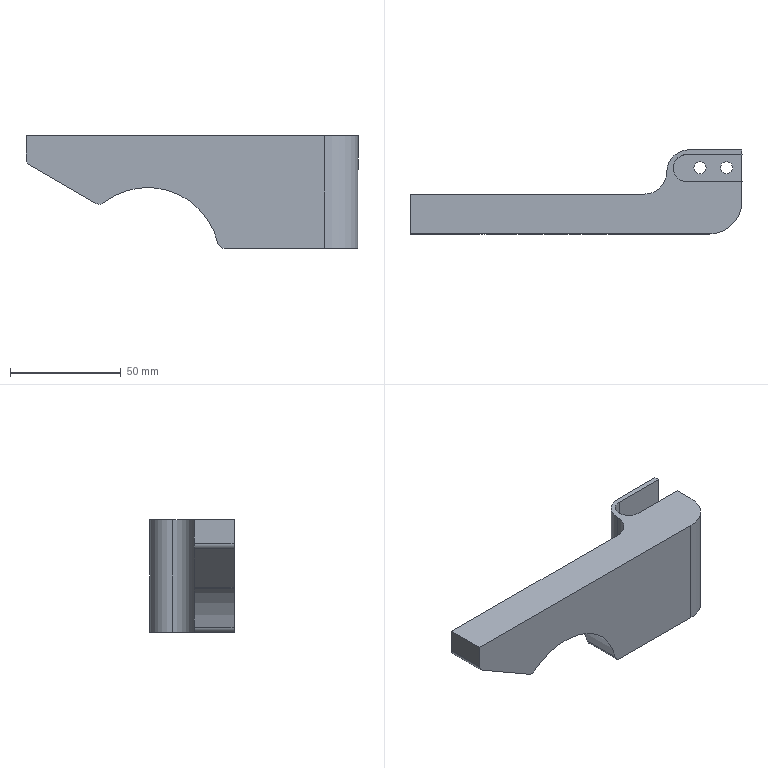CAM job | NX | 3-axis milling, drilling | part box 150 x 38 x 51 mm | stock box 160 x 48 x 52 mm
Tools:
number,name,description,diameter,corner_radius,flute_length,length,flutes
1,D63,Milling Tool-5 Parameters,63.0,0.0,50.0,75.0,2
12,D12C,Milling Tool-5 Parameters,12.0,0.0,50.0,75.0,2
8,R4,Milling Tool-5 Parameters,8.0,4.0,50.0,75.0,2
7,D6A45,Milling Tool-5 Parameters,6.0,0.0,50.0,75.0,2
15,5.5ZT,Drilling Tool,5.5,0.0,35.0,50.0,2
6,D6,Milling Tool-5 Parameters,6.0,0.0,50.0,75.0,2
11,D12JING,Milling Tool-5 Parameters,12.0,0.0,50.0,75.0,2
Operations:
program,operation,operation_type,tool,method,geometry_group,spindle_rpm,surface_speed,feed_per_tooth,feed_cut,feed_plunge,cut_length_mm,path_length_mm,cut_time_min,machine_time_min
1,FLOOR_WALL,VolumeBased25DMillingOperation,D63,METHOD,A,6500.0,1286.0,0.1154,1500.0,100.0,480.797,534.797,0.3205,0.3259
1,DRILLING,Operation,D6A45,METHOD,A,5000.0,94.0,0.025,250.0,0.0,8.0,91.369,0.032,0.0403
1,DRILLING_COPY,Operation,5.5ZT,METHOD,A,2000.0,34.0,0.05,200.0,0.0,89.305,253.979,0.4465,0.463
1,ADAPTIVE_MILLING,CavityMilling,D12C,METHOD,A,9500.0,358.0,0.1579,3000.0,1000.0,5698.893,5804.893,1.902,1.912
1,ADAPTIVE_MILLING_COPY,CavityMilling,D12C,METHOD,A,9500.0,358.0,0.1579,3000.0,1000.0,5696.238,5852.238,1.901,1.916
1,CAVITY_MILL,CavityMilling,D12C,METHOD,A,9500.0,358.0,0.1316,2500.0,1000.0,10840.921,11390.241,4.866,4.921
1,ZLEVEL_PROFILE_COPY_COPY_COPY_1_COPY_COPY_COPY,ZLevelMilling,D12JING,METHOD,A,9500.0,358.0,0.0632,1200.0,1000.0,1630.857,1796.09,1.362,1.378
1,HOLE_MILLING,CylinderMilling,D6,METHOD,A,9500.0,179.0,0.0447,850.0,100.0,2649.12,2831.72,3.117,3.135
1,PLANAR_MILL,PlanarMilling,D6A45,METHOD,A,9500.0,179.0,0.0658,1250.0,100.0,238.269,490.876,0.1906,0.2159
1,FIXED_CONTOUR,SurfaceContour,R4,METHOD,A,9500.0,119.0,0.1579,3000.0,100.0,24000.136,24098.242,8.0,8.01